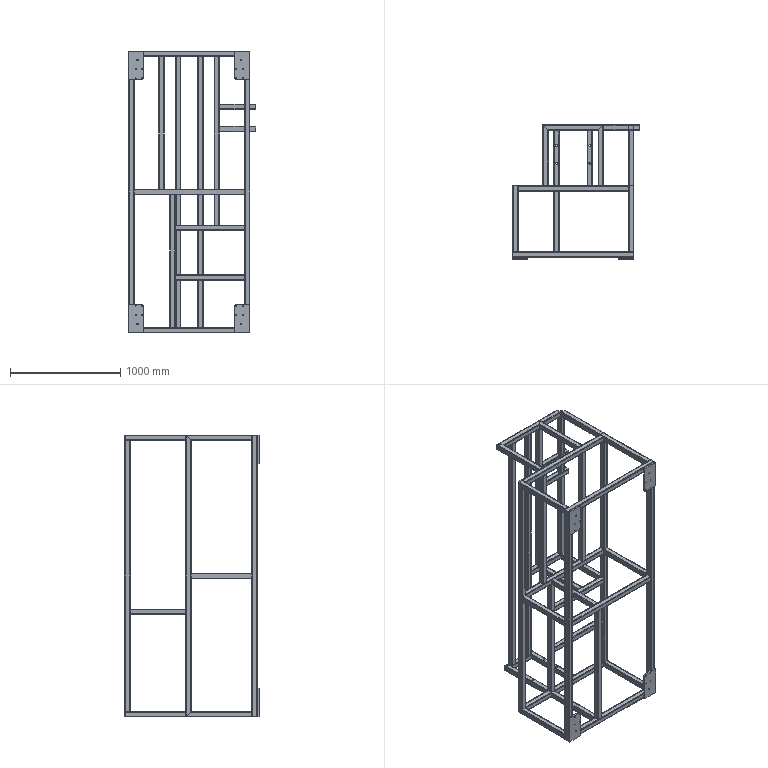Part | STEP file | 44 solids | 868 faces | box 1150 x 1215 x 2550 mm | volume 25178560 mm3 | plane 460 | cylinder 408 | commonest cylinder face diameters 6.4 x176 12.8 x176 6.8 x32 17 x16 14 x8